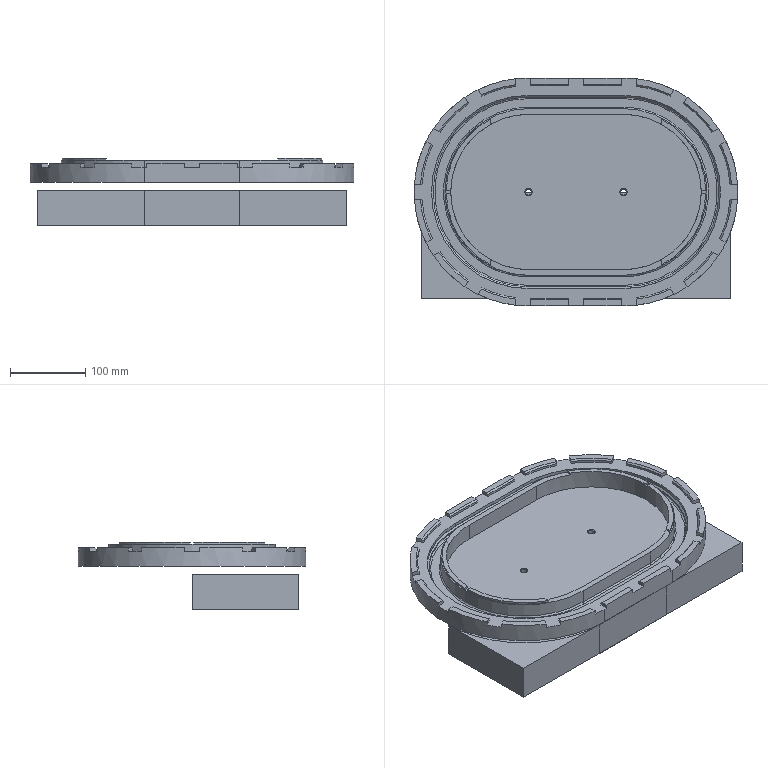CAM job | NX | 3-axis milling, drilling | part box 429 x 302 x 89.371 mm
Tools:
number,name,description,diameter,corner_radius,flute_length,length,flutes
2,D16开粗,Milling Tool-5 Parameters,16.0,0.0,50.0,75.0,2
2,D8平刀,Milling Tool-5 Parameters,8.0,0.0,50.0,75.0,2
1,D63.,Milling Tool-5 Parameters,63.0,0.0,50.0,75.0,2
4,钻头10.5,Drilling Tool,10.5,0.0,35.0,50.0,2
3,倒角12.,Drilling Tool,12.0,0.0,35.0,50.0,2
3,D16精光,Milling Tool-5 Parameters,16.0,0.0,50.0,75.0,2
5,倒角-6.,Drilling Tool,6.0,0.0,35.0,50.0,2
4,D10R1,Milling Tool-5 Parameters,10.0,1.0,20.0,50.0,4
Operations:
program,operation,operation_type,tool,method,geometry_group,spindle_rpm,surface_speed,feed_per_tooth,feed_cut,feed_plunge,cut_length_mm,path_length_mm,cut_time_min,machine_time_min
G54,ADAPTIVE_MILLING,CavityMilling,D16开粗,METHOD,G54,6500.0,326.0,0.2308,3000.0,100.0,140022.756,154572.543,44.872,46.327
G54,ADAPTIVE_MILLING_COPY,CavityMilling,D8平刀,METHOD,G54,6500.0,326.0,0.2308,3000.0,100.0,31896.559,48452.618,10.625,12.281
PROGRAM_1,PLANAR_MILL,PlanarMilling,D63.,METHOD,WORKPIECE,4500.0,890.0,0.1667,1500.0,100.0,659.044,752.844,0.4394,0.4487
PROGRAM_1,ADAPTIVE_MILLING_2,CavityMilling,D16开粗,METHOD,WORKPIECE_1,6500.0,326.0,0.2308,3000.0,100.0,14544.118,15178.772,4.809,4.873
PROGRAM_1,PLANAR_MILL_2_COPY,PlanarMilling,D16开粗,METHOD,WORKPIECE_1,5500.0,276.0,0.0727,800.0,100.0,655.166,849.466,0.819,0.8384
PROGRAM_1,PLANAR_MILL_COPY,PlanarMilling,D63.,METHOD,WORKPIECE,4500.0,890.0,0.0778,700.0,100.0,659.044,753.044,0.9415,0.9509
PROGRAM_2,PLANAR_MILL_2,PlanarMilling,D16开粗,METHOD,WORKPIECE_1,6500.0,326.0,0.2692,3500.0,100.0,20084.687,39609.684,5.739,7.691
PROGRAM_2,PLANAR_MILL_2_COPY_2,PlanarMilling,D16开粗,METHOD,WORKPIECE_1,6500.0,326.0,0.2308,3000.0,100.0,12720.14,24049.426,4.24,5.373
PROGRAM_2,PLANAR_MILL_2_COPY_2_COPY,PlanarMilling,D16开粗,METHOD,WORKPIECE_1,6500.0,326.0,0.2692,800.0,100.0,544.32,686.091,0.6804,0.6946
PROGRAM_2,PLANAR_MILL_2_COPY_1,PlanarMilling,D16开粗,METHOD,WORKPIECE_1,6500.0,326.0,0.0615,800.0,100.0,590.726,784.626,0.7384,0.7578
FIXTURE,FLOOR_FACING,VolumeBased25DMillingOperation,D63.,METHOD,WORKPIECE_2,4500.0,890.0,0.1667,1500.0,100.0,1763.256,4038.941,1.175,1.403
FIXTURE,DRILLING_COPY,Operation,倒角12.,METHOD,WORKPIECE_2,1500.0,56.0,0.05,150.0,0.0,34.0,525.92,0.2267,0.2759
FIXTURE,DRILLING,Operation,钻头10.5,METHOD,WORKPIECE_2,1200.0,39.0,0.075,180.0,0.0,240.0,937.92,1.333,1.403
FIXTURE,DRILLING_COPY_1,Operation,D16开粗,METHOD,WORKPIECE_2,700.0,35.0,0.0857,120.0,0.0,72.0,601.92,0.6,0.653
FINISH,PLANAR_MILL_COPY_1,PlanarMilling,D63.,METHOD,FINISH.,4500.0,890.0,0.1667,1500.0,100.0,659.044,752.844,0.4394,0.4487
FINISH,PLANAR_MILL_2_COPY_2_COPY_1,PlanarMilling,D16开粗,METHOD,FINISH.,6500.0,326.0,0.2308,3000.0,100.0,10476.621,18336.791,3.492,4.278
FINISH,PLANAR_MILL_2_COPY_3,PlanarMilling,D16开粗,METHOD,FINISH.,6500.0,326.0,0.2692,3500.0,100.0,9451.617,18723.189,2.7,3.628
FINISH,CURVE_DRIVE,SurfaceContour,D16开粗,METHOD,FINISH.,5000.0,251.0,0.3,3000.0,100.0,7007.63,7151.63,2.336,2.35
FINISH,PLANAR_MILL_2_COPY_COPY,PlanarMilling,D16开粗,METHOD,FINISH.,6500.0,326.0,0.2308,3000.0,100.0,20764.346,38541.165,6.921,8.699
FINISH,PLANAR_MILL_2_COPY_2_COPY_1_COPY,PlanarMilling,D16精光,METHOD,FINISH.,5500.0,276.0,0.0727,800.0,100.0,1073.734,1738.061,1.342,1.409
FINISH,PLANAR_MILL_2_COPY_3_COPY,PlanarMilling,D16精光,METHOD,FINISH.,5500.0,276.0,0.0727,800.0,100.0,1181.452,1998.252,1.477,1.558
FINISH,PLANAR_MILL_2_COPY_COPY_COPY,PlanarMilling,D16精光,METHOD,FINISH.,5500.0,276.0,0.0727,800.0,100.0,1297.159,2098.345,1.621,1.702
FINISH,CURVE_DRIVE_COPY,SurfaceContour,D10R1,METHOD,FINISH.,6500.0,100.0,0.1178,3500.0,100.0,32116.692,32262.692,9.176,9.191
FINISH,PLANAR_MILL_2_COPY_2_COPY_1_COPY_COPY,PlanarMilling,倒角-6.,METHOD,FINISH.,5500.0,276.0,0.0727,800.0,100.0,1146.451,1244.451,1.433,1.443
FINISH,PLANAR_MILL_COPY_COPY,PlanarMilling,D63.,METHOD,FINISH.,4500.0,890.0,0.0778,700.0,100.0,659.044,753.044,0.9415,0.9509
FINISH,PLANAR_MILL_2_COPY_3_COPY_COPY,PlanarMilling,D16精光,METHOD,FINISH.,5500.0,276.0,0.0727,800.0,100.0,590.726,784.326,0.7384,0.7578
FINISH,PLANAR_MILL_2_COPY_COPY_COPY_COPY,PlanarMilling,D16精光,METHOD,FINISH.,5500.0,276.0,0.0727,800.0,100.0,649.2,842.8,0.8115,0.8309
CHAMFER.,PLANAR_MILL_2_COPY_2_COPY_1_COPY_COPY_COPY,PlanarMilling,倒角-6.,METHOD,CHAMFER.,5500.0,103.0,0.1091,1200.0,100.0,1626.785,2678.776,1.356,1.461